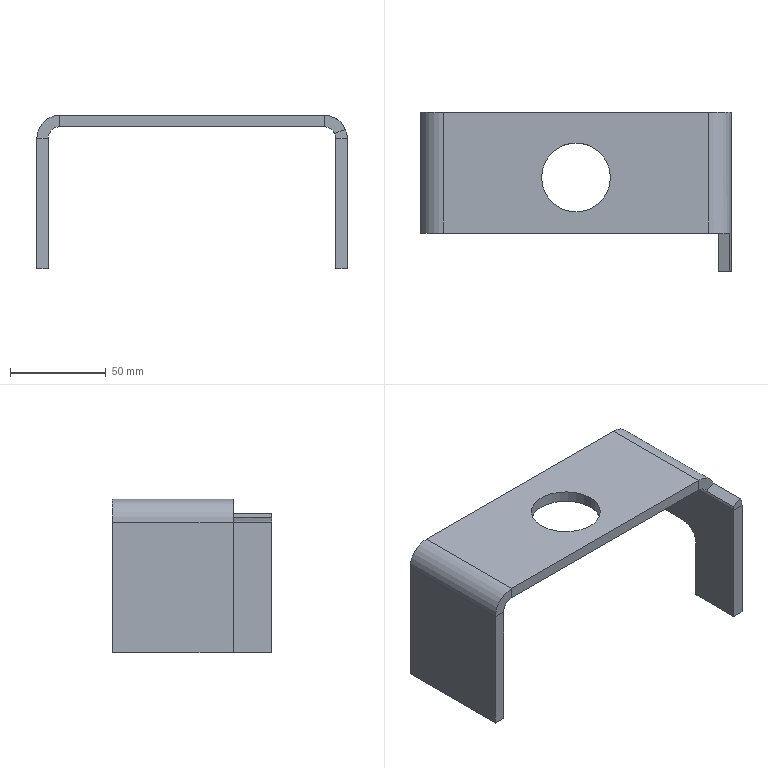Part | SolidWorks | features ICE 3, Fillet 1, FlatPattern 1, SMBaseFlange 1, SheetMetal 1 | 1 solid | 29 faces | box 162 x 83 x 80 mm | volume 102695 mm3 | plane 22 | cylinder 7 | commonest cylinder face diameters 12 x2 24 x2 36 x2 20 x1
STEP:
#1=CARTESIAN_POINT('',(63.,49.,-6.));
#2=VERTEX_POINT('',#1);
#3=CARTESIAN_POINT('',(99.,49.,-6.));
#4=VERTEX_POINT('',#3);
#5=CARTESIAN_POINT('',(81.,49.,-6.));
#6=DIRECTION('',(0.,0.,1.));
#7=DIRECTION('',(1.,0.,0.));
#8=AXIS2_PLACEMENT_3D('',#5,#6,#7);
#9=CIRCLE('',#8,18.);
#10=EDGE_CURVE('',#2,#4,#9,.T.);
#11=ORIENTED_EDGE('',*,*,#10,.F.);
#12=CARTESIAN_POINT('',(63.,49.,0.));
#13=VERTEX_POINT('',#12);
#14=CARTESIAN_POINT('',(63.,49.,-6.));
#15=DIRECTION('',(0.,0.,1.));
#16=VECTOR('',#15,1000.);
#17=LINE('',#14,#16);
#18=EDGE_CURVE('',#2,#13,#17,.T.);
#19=ORIENTED_EDGE('',*,*,#18,.T.);
#20=CARTESIAN_POINT('',(99.,49.,0.));
#21=VERTEX_POINT('',#20);
#22=CARTESIAN_POINT('',(81.,49.,0.));
#23=DIRECTION('',(0.,0.,1.));
#24=DIRECTION('',(1.,0.,0.));
#25=AXIS2_PLACEMENT_3D('',#22,#23,#24);
#26=CIRCLE('',#25,18.);
#27=EDGE_CURVE('',#13,#21,#26,.T.);
#28=ORIENTED_EDGE('',*,*,#27,.T.);
#29=CARTESIAN_POINT('',(99.,49.,-6.));
#30=DIRECTION('',(0.,0.,1.));
#31=VECTOR('',#30,1000.);
#32=LINE('',#29,#31);
#33=EDGE_CURVE('',#4,#21,#32,.T.);
#34=ORIENTED_EDGE('',*,*,#33,.F.);
#35=EDGE_LOOP('',(#11,#19,#28,#34));
#36=FACE_OUTER_BOUND('',#35,.T.);
#37=CARTESIAN_POINT('',(81.,49.,-6.));
#38=DIRECTION('',(0.,0.,1.));
#39=DIRECTION('',(1.,0.,0.));
#40=AXIS2_PLACEMENT_3D('',#37,#38,#39);
#41=CYLINDRICAL_SURFACE('',#40,18.);
#42=ADVANCED_FACE('',(#36),#41,.F.);
#43=CARTESIAN_POINT('',(161.,0.,-7.204));
#44=VERTEX_POINT('',#43);
#45=CARTESIAN_POINT('',(162.,0.,-12.));
#46=VERTEX_POINT('',#45);
#47=CARTESIAN_POINT('',(150.,0.,-12.));
#48=DIRECTION('',(0.,1.,0.));
#49=DIRECTION('',(0.,0.,-1.));
#50=AXIS2_PLACEMENT_3D('',#47,#48,#49);
#51=CIRCLE('',#50,12.);
#52=EDGE_CURVE('',#44,#46,#51,.T.);
#53=ORIENTED_EDGE('',*,*,#52,.F.);
#54=CARTESIAN_POINT('',(155.5,0.,-9.602));
#55=VERTEX_POINT('',#54);
#56=CARTESIAN_POINT('',(155.5,0.,-9.602));
#57=DIRECTION('',(0.9167,0.,0.3997));
#58=VECTOR('',#57,1000.);
#59=LINE('',#56,#58);
#60=EDGE_CURVE('',#55,#44,#59,.T.);
#61=ORIENTED_EDGE('',*,*,#60,.F.);
#62=CARTESIAN_POINT('',(156.,0.,-12.));
#63=VERTEX_POINT('',#62);
#64=CARTESIAN_POINT('',(150.,0.,-12.));
#65=DIRECTION('',(0.,1.,0.));
#66=DIRECTION('',(1.,0.,0.));
#67=AXIS2_PLACEMENT_3D('',#64,#65,#66);
#68=CIRCLE('',#67,6.);
#69=EDGE_CURVE('',#55,#63,#68,.T.);
#70=ORIENTED_EDGE('',*,*,#69,.T.);
#71=CARTESIAN_POINT('',(162.,0.,-12.));
#72=DIRECTION('',(-1.,0.,0.));
#73=VECTOR('',#72,1000.);
#74=LINE('',#71,#73);
#75=EDGE_CURVE('',#46,#63,#74,.T.);
#76=ORIENTED_EDGE('',*,*,#75,.F.);
#77=EDGE_LOOP('',(#53,#61,#70,#76));
#78=FACE_OUTER_BOUND('',#77,.T.);
#79=CARTESIAN_POINT('',(162.,0.,-12.));
#80=DIRECTION('',(0.,-1.,0.));
#81=DIRECTION('',(0.,0.,-1.));
#82=AXIS2_PLACEMENT_3D('',#79,#80,#81);
#83=PLANE('',#82);
#84=ADVANCED_FACE('',(#78),#83,.T.);
#85=CARTESIAN_POINT('',(155.5,20.,-9.602));
#86=VERTEX_POINT('',#85);
#87=CARTESIAN_POINT('',(155.5,83.,-9.602));
#88=DIRECTION('',(0.,-1.,0.));
#89=VECTOR('',#88,1000.);
#90=LINE('',#87,#89);
#91=EDGE_CURVE('',#86,#55,#90,.T.);
#92=ORIENTED_EDGE('',*,*,#91,.F.);
#93=CARTESIAN_POINT('',(150.,20.,-6.));
#94=VERTEX_POINT('',#93);
#95=CARTESIAN_POINT('',(150.,20.,-12.));
#96=DIRECTION('',(0.,-1.,0.));
#97=DIRECTION('',(0.,0.,-1.));
#98=AXIS2_PLACEMENT_3D('',#95,#96,#97);
#99=CIRCLE('',#98,6.);
#100=EDGE_CURVE('',#86,#94,#99,.T.);
#101=ORIENTED_EDGE('',*,*,#100,.T.);
#102=CARTESIAN_POINT('',(150.,83.,-6.));
#103=VERTEX_POINT('',#102);
#104=CARTESIAN_POINT('',(150.,83.,-6.));
#105=DIRECTION('',(0.,-1.,0.));
#106=VECTOR('',#105,1000.);
#107=LINE('',#104,#106);
#108=EDGE_CURVE('',#103,#94,#107,.T.);
#109=ORIENTED_EDGE('',*,*,#108,.F.);
#110=CARTESIAN_POINT('',(156.,83.,-12.));
#111=VERTEX_POINT('',#110);
#112=CARTESIAN_POINT('',(150.,83.,-12.));
#113=DIRECTION('',(0.,1.,0.));
#114=DIRECTION('',(1.,0.,0.));
#115=AXIS2_PLACEMENT_3D('',#112,#113,#114);
#116=CIRCLE('',#115,6.);
#117=EDGE_CURVE('',#103,#111,#116,.T.);
#118=ORIENTED_EDGE('',*,*,#117,.T.);
#119=CARTESIAN_POINT('',(156.,83.,-12.));
#120=DIRECTION('',(0.,-1.,0.));
#121=VECTOR('',#120,1000.);
#122=LINE('',#119,#121);
#123=EDGE_CURVE('',#111,#63,#122,.T.);
#124=ORIENTED_EDGE('',*,*,#123,.T.);
#125=ORIENTED_EDGE('',*,*,#69,.F.);
#126=EDGE_LOOP('',(#92,#101,#109,#118,#124,#125));
#127=FACE_OUTER_BOUND('',#126,.T.);
#128=CARTESIAN_POINT('',(150.,83.,-12.));
#129=DIRECTION('',(0.,-1.,0.));
#130=DIRECTION('',(0.,0.,-1.));
#131=AXIS2_PLACEMENT_3D('',#128,#129,#130);
#132=CYLINDRICAL_SURFACE('',#131,6.);
#133=ADVANCED_FACE('',(#127),#132,.F.);
#134=CARTESIAN_POINT('',(81.,49.,-6.));
#135=DIRECTION('',(0.,0.,1.));
#136=DIRECTION('',(1.,0.,0.));
#137=AXIS2_PLACEMENT_3D('',#134,#135,#136);
#138=CIRCLE('',#137,18.);
#139=EDGE_CURVE('',#4,#2,#138,.T.);
#140=ORIENTED_EDGE('',*,*,#139,.T.);
#141=ORIENTED_EDGE('',*,*,#10,.T.);
#142=EDGE_LOOP('',(#140,#141));
#143=FACE_BOUND('',#142,.T.);
#144=ORIENTED_EDGE('',*,*,#108,.T.);
#145=CARTESIAN_POINT('',(12.,20.,-6.));
#146=VERTEX_POINT('',#145);
#147=CARTESIAN_POINT('',(0.,20.,-6.));
#148=DIRECTION('',(-1.,0.,0.));
#149=VECTOR('',#148,1000.);
#150=LINE('',#147,#149);
#151=EDGE_CURVE('',#94,#146,#150,.T.);
#152=ORIENTED_EDGE('',*,*,#151,.T.);
#153=CARTESIAN_POINT('',(12.,83.,-6.));
#154=VERTEX_POINT('',#153);
#155=CARTESIAN_POINT('',(12.,83.,-6.));
#156=DIRECTION('',(0.,-1.,0.));
#157=VECTOR('',#156,1000.);
#158=LINE('',#155,#157);
#159=EDGE_CURVE('',#154,#146,#158,.T.);
#160=ORIENTED_EDGE('',*,*,#159,.F.);
#161=CARTESIAN_POINT('',(0.,83.,-6.));
#162=DIRECTION('',(1.,0.,0.));
#163=VECTOR('',#162,1000.);
#164=LINE('',#161,#163);
#165=EDGE_CURVE('',#154,#103,#164,.T.);
#166=ORIENTED_EDGE('',*,*,#165,.T.);
#167=EDGE_LOOP('',(#144,#152,#160,#166));
#168=FACE_OUTER_BOUND('',#167,.T.);
#169=CARTESIAN_POINT('',(0.,83.,-6.));
#170=DIRECTION('',(0.,0.,-1.));
#171=DIRECTION('',(-1.,0.,0.));
#172=AXIS2_PLACEMENT_3D('',#169,#170,#171);
#173=PLANE('',#172);
#174=ADVANCED_FACE('',(#143,#168),#173,.T.);
#175=ORIENTED_EDGE('',*,*,#159,.T.);
#176=CARTESIAN_POINT('',(6.,20.,-12.));
#177=VERTEX_POINT('',#176);
#178=CARTESIAN_POINT('',(12.,20.,-12.));
#179=DIRECTION('',(0.,-1.,0.));
#180=DIRECTION('',(0.,0.,-1.));
#181=AXIS2_PLACEMENT_3D('',#178,#179,#180);
#182=CIRCLE('',#181,6.);
#183=EDGE_CURVE('',#146,#177,#182,.T.);
#184=ORIENTED_EDGE('',*,*,#183,.T.);
#185=CARTESIAN_POINT('',(6.,83.,-12.));
#186=VERTEX_POINT('',#185);
#187=CARTESIAN_POINT('',(6.,83.,-12.));
#188=DIRECTION('',(0.,-1.,0.));
#189=VECTOR('',#188,1000.);
#190=LINE('',#187,#189);
#191=EDGE_CURVE('',#186,#177,#190,.T.);
#192=ORIENTED_EDGE('',*,*,#191,.F.);
#193=CARTESIAN_POINT('',(12.,83.,-12.));
#194=DIRECTION('',(0.,1.,0.));
#195=DIRECTION('',(1.,0.,0.));
#196=AXIS2_PLACEMENT_3D('',#193,#194,#195);
#197=CIRCLE('',#196,6.);
#198=EDGE_CURVE('',#186,#154,#197,.T.);
#199=ORIENTED_EDGE('',*,*,#198,.T.);
#200=EDGE_LOOP('',(#175,#184,#192,#199));
#201=FACE_OUTER_BOUND('',#200,.T.);
#202=CARTESIAN_POINT('',(12.,83.,-12.));
#203=DIRECTION('',(0.,-1.,0.));
#204=DIRECTION('',(0.,0.,-1.));
#205=AXIS2_PLACEMENT_3D('',#202,#203,#204);
#206=CYLINDRICAL_SURFACE('',#205,6.);
#207=ADVANCED_FACE('',(#201),#206,.F.);
#208=ORIENTED_EDGE('',*,*,#191,.T.);
#209=CARTESIAN_POINT('',(6.,20.,-80.));
#210=VERTEX_POINT('',#209);
#211=CARTESIAN_POINT('',(6.,20.,-80.));
#212=DIRECTION('',(0.,0.,-1.));
#213=VECTOR('',#212,1000.);
#214=LINE('',#211,#213);
#215=EDGE_CURVE('',#177,#210,#214,.T.);
#216=ORIENTED_EDGE('',*,*,#215,.T.);
#217=CARTESIAN_POINT('',(6.,83.,-80.));
#218=VERTEX_POINT('',#217);
#219=CARTESIAN_POINT('',(6.,83.,-80.));
#220=DIRECTION('',(0.,-1.,0.));
#221=VECTOR('',#220,1000.);
#222=LINE('',#219,#221);
#223=EDGE_CURVE('',#218,#210,#222,.T.);
#224=ORIENTED_EDGE('',*,*,#223,.F.);
#225=CARTESIAN_POINT('',(6.,83.,-80.));
#226=DIRECTION('',(0.,0.,1.));
#227=VECTOR('',#226,1000.);
#228=LINE('',#225,#227);
#229=EDGE_CURVE('',#218,#186,#228,.T.);
#230=ORIENTED_EDGE('',*,*,#229,.T.);
#231=EDGE_LOOP('',(#208,#216,#224,#230));
#232=FACE_OUTER_BOUND('',#231,.T.);
#233=CARTESIAN_POINT('',(6.,83.,-80.));
#234=DIRECTION('',(1.,0.,0.));
#235=DIRECTION('',(0.,0.,-1.));
#236=AXIS2_PLACEMENT_3D('',#233,#234,#235);
#237=PLANE('',#236);
#238=ADVANCED_FACE('',(#232),#237,.T.);
#239=ORIENTED_EDGE('',*,*,#223,.T.);
#240=CARTESIAN_POINT('',(0.,20.,-80.));
#241=VERTEX_POINT('',#240);
#242=CARTESIAN_POINT('',(6.,20.,-80.));
#243=DIRECTION('',(-1.,0.,0.));
#244=VECTOR('',#243,1000.);
#245=LINE('',#242,#244);
#246=EDGE_CURVE('',#210,#241,#245,.T.);
#247=ORIENTED_EDGE('',*,*,#246,.T.);
#248=CARTESIAN_POINT('',(0.,83.,-80.));
#249=VERTEX_POINT('',#248);
#250=CARTESIAN_POINT('',(0.,83.,-80.));
#251=DIRECTION('',(0.,-1.,0.));
#252=VECTOR('',#251,1000.);
#253=LINE('',#250,#252);
#254=EDGE_CURVE('',#249,#241,#253,.T.);
#255=ORIENTED_EDGE('',*,*,#254,.F.);
#256=CARTESIAN_POINT('',(0.,83.,-80.));
#257=DIRECTION('',(1.,0.,0.));
#258=VECTOR('',#257,1000.);
#259=LINE('',#256,#258);
#260=EDGE_CURVE('',#249,#218,#259,.T.);
#261=ORIENTED_EDGE('',*,*,#260,.T.);
#262=EDGE_LOOP('',(#239,#247,#255,#261));
#263=FACE_OUTER_BOUND('',#262,.T.);
#264=CARTESIAN_POINT('',(0.,83.,-80.));
#265=DIRECTION('',(0.,0.,-1.));
#266=DIRECTION('',(-1.,0.,0.));
#267=AXIS2_PLACEMENT_3D('',#264,#265,#266);
#268=PLANE('',#267);
#269=ADVANCED_FACE('',(#263),#268,.T.);
#270=CARTESIAN_POINT('',(0.,20.,-12.));
#271=VERTEX_POINT('',#270);
#272=CARTESIAN_POINT('',(0.,20.,-80.));
#273=DIRECTION('',(0.,0.,-1.));
#274=VECTOR('',#273,1000.);
#275=LINE('',#272,#274);
#276=EDGE_CURVE('',#271,#241,#275,.T.);
#277=ORIENTED_EDGE('',*,*,#276,.F.);
#278=CARTESIAN_POINT('',(0.,83.,-12.));
#279=VERTEX_POINT('',#278);
#280=CARTESIAN_POINT('',(0.,83.,-12.));
#281=DIRECTION('',(0.,-1.,0.));
#282=VECTOR('',#281,1000.);
#283=LINE('',#280,#282);
#284=EDGE_CURVE('',#279,#271,#283,.T.);
#285=ORIENTED_EDGE('',*,*,#284,.F.);
#286=CARTESIAN_POINT('',(0.,83.,-80.));
#287=DIRECTION('',(0.,0.,1.));
#288=VECTOR('',#287,1000.);
#289=LINE('',#286,#288);
#290=EDGE_CURVE('',#249,#279,#289,.T.);
#291=ORIENTED_EDGE('',*,*,#290,.F.);
#292=ORIENTED_EDGE('',*,*,#254,.T.);
#293=EDGE_LOOP('',(#277,#285,#291,#292));
#294=FACE_OUTER_BOUND('',#293,.T.);
#295=CARTESIAN_POINT('',(0.,83.,-80.));
#296=DIRECTION('',(1.,0.,0.));
#297=DIRECTION('',(0.,0.,-1.));
#298=AXIS2_PLACEMENT_3D('',#295,#296,#297);
#299=PLANE('',#298);
#300=ADVANCED_FACE('',(#294),#299,.F.);
#301=CARTESIAN_POINT('',(12.,20.,0.));
#302=VERTEX_POINT('',#301);
#303=CARTESIAN_POINT('',(12.,20.,-12.));
#304=DIRECTION('',(0.,-1.,0.));
#305=DIRECTION('',(0.,0.,-1.));
#306=AXIS2_PLACEMENT_3D('',#303,#304,#305);
#307=CIRCLE('',#306,12.);
#308=EDGE_CURVE('',#302,#271,#307,.T.);
#309=ORIENTED_EDGE('',*,*,#308,.F.);
#310=CARTESIAN_POINT('',(12.,83.,0.));
#311=VERTEX_POINT('',#310);
#312=CARTESIAN_POINT('',(12.,83.,0.));
#313=DIRECTION('',(0.,-1.,0.));
#314=VECTOR('',#313,1000.);
#315=LINE('',#312,#314);
#316=EDGE_CURVE('',#311,#302,#315,.T.);
#317=ORIENTED_EDGE('',*,*,#316,.F.);
#318=CARTESIAN_POINT('',(12.,83.,-12.));
#319=DIRECTION('',(0.,1.,0.));
#320=DIRECTION('',(0.,0.,-1.));
#321=AXIS2_PLACEMENT_3D('',#318,#319,#320);
#322=CIRCLE('',#321,12.);
#323=EDGE_CURVE('',#279,#311,#322,.T.);
#324=ORIENTED_EDGE('',*,*,#323,.F.);
#325=ORIENTED_EDGE('',*,*,#284,.T.);
#326=EDGE_LOOP('',(#309,#317,#324,#325));
#327=FACE_OUTER_BOUND('',#326,.T.);
#328=CARTESIAN_POINT('',(12.,83.,-12.));
#329=DIRECTION('',(0.,-1.,0.));
#330=DIRECTION('',(0.,0.,-1.));
#331=AXIS2_PLACEMENT_3D('',#328,#329,#330);
#332=CYLINDRICAL_SURFACE('',#331,12.);
#333=ADVANCED_FACE('',(#327),#332,.T.);
#334=CARTESIAN_POINT('',(81.,49.,0.));
#335=DIRECTION('',(0.,0.,1.));
#336=DIRECTION('',(1.,0.,0.));
#337=AXIS2_PLACEMENT_3D('',#334,#335,#336);
#338=CIRCLE('',#337,18.);
#339=EDGE_CURVE('',#21,#13,#338,.T.);
#340=ORIENTED_EDGE('',*,*,#339,.F.);
#341=ORIENTED_EDGE('',*,*,#27,.F.);
#342=EDGE_LOOP('',(#340,#341));
#343=FACE_BOUND('',#342,.T.);
#344=CARTESIAN_POINT('',(150.,20.,0.));
#345=VERTEX_POINT('',#344);
#346=CARTESIAN_POINT('',(0.,20.,0.));
#347=DIRECTION('',(-1.,0.,0.));
#348=VECTOR('',#347,1000.);
#349=LINE('',#346,#348);
#350=EDGE_CURVE('',#345,#302,#349,.T.);
#351=ORIENTED_EDGE('',*,*,#350,.F.);
#352=CARTESIAN_POINT('',(150.,83.,0.));
#353=VERTEX_POINT('',#352);
#354=CARTESIAN_POINT('',(150.,83.,0.));
#355=DIRECTION('',(0.,-1.,0.));
#356=VECTOR('',#355,1000.);
#357=LINE('',#354,#356);
#358=EDGE_CURVE('',#353,#345,#357,.T.);
#359=ORIENTED_EDGE('',*,*,#358,.F.);
#360=CARTESIAN_POINT('',(0.,83.,0.));
#361=DIRECTION('',(1.,0.,0.));
#362=VECTOR('',#361,1000.);
#363=LINE('',#360,#362);
#364=EDGE_CURVE('',#311,#353,#363,.T.);
#365=ORIENTED_EDGE('',*,*,#364,.F.);
#366=ORIENTED_EDGE('',*,*,#316,.T.);
#367=EDGE_LOOP('',(#351,#359,#365,#366));
#368=FACE_OUTER_BOUND('',#367,.T.);
#369=CARTESIAN_POINT('',(0.,83.,0.));
#370=DIRECTION('',(0.,0.,-1.));
#371=DIRECTION('',(-1.,0.,0.));
#372=AXIS2_PLACEMENT_3D('',#369,#370,#371);
#373=PLANE('',#372);
#374=ADVANCED_FACE('',(#343,#368),#373,.F.);
#375=CARTESIAN_POINT('',(161.,20.,-7.204));
#376=VERTEX_POINT('',#375);
#377=CARTESIAN_POINT('',(150.,20.,-12.));
#378=DIRECTION('',(0.,-1.,0.));
#379=DIRECTION('',(0.,0.,-1.));
#380=AXIS2_PLACEMENT_3D('',#377,#378,#379);
#381=CIRCLE('',#380,12.);
#382=EDGE_CURVE('',#376,#345,#381,.T.);
#383=ORIENTED_EDGE('',*,*,#382,.F.);
#384=CARTESIAN_POINT('',(161.,83.,-7.204));
#385=DIRECTION('',(0.,-1.,0.));
#386=VECTOR('',#385,1000.);
#387=LINE('',#384,#386);
#388=EDGE_CURVE('',#376,#44,#387,.T.);
#389=ORIENTED_EDGE('',*,*,#388,.T.);
#390=ORIENTED_EDGE('',*,*,#52,.T.);
#391=CARTESIAN_POINT('',(162.,83.,-12.));
#392=VERTEX_POINT('',#391);
#393=CARTESIAN_POINT('',(162.,83.,-12.));
#394=DIRECTION('',(0.,-1.,0.));
#395=VECTOR('',#394,1000.);
#396=LINE('',#393,#395);
#397=EDGE_CURVE('',#392,#46,#396,.T.);
#398=ORIENTED_EDGE('',*,*,#397,.F.);
#399=CARTESIAN_POINT('',(150.,83.,-12.));
#400=DIRECTION('',(0.,1.,0.));
#401=DIRECTION('',(0.,0.,-1.));
#402=AXIS2_PLACEMENT_3D('',#399,#400,#401);
#403=CIRCLE('',#402,12.);
#404=EDGE_CURVE('',#353,#392,#403,.T.);
#405=ORIENTED_EDGE('',*,*,#404,.F.);
#406=ORIENTED_EDGE('',*,*,#358,.T.);
#407=EDGE_LOOP('',(#383,#389,#390,#398,#405,#406));
#408=FACE_OUTER_BOUND('',#407,.T.);
#409=CARTESIAN_POINT('',(150.,83.,-12.));
#410=DIRECTION('',(0.,-1.,0.));
#411=DIRECTION('',(0.,0.,-1.));
#412=AXIS2_PLACEMENT_3D('',#409,#410,#411);
#413=CYLINDRICAL_SURFACE('',#412,12.);
#414=ADVANCED_FACE('',(#408),#413,.T.);
#415=CARTESIAN_POINT('',(0.,83.,-12.));
#416=DIRECTION('',(1.,0.,0.));
#417=VECTOR('',#416,1000.);
#418=LINE('',#415,#417);
#419=EDGE_CURVE('',#279,#186,#418,.T.);
#420=ORIENTED_EDGE('',*,*,#419,.F.);
#421=ORIENTED_EDGE('',*,*,#323,.T.);
#422=CARTESIAN_POINT('',(12.,83.,-6.));
#423=DIRECTION('',(0.,0.,1.));
#424=VECTOR('',#423,1000.);
#425=LINE('',#422,#424);
#426=EDGE_CURVE('',#154,#311,#425,.T.);
#427=ORIENTED_EDGE('',*,*,#426,.F.);
#428=ORIENTED_EDGE('',*,*,#198,.F.);
#429=EDGE_LOOP('',(#420,#421,#427,#428));
#430=FACE_OUTER_BOUND('',#429,.T.);
#431=CARTESIAN_POINT('',(0.,83.,-12.));
#432=DIRECTION('',(0.,1.,0.));
#433=DIRECTION('',(0.,0.,1.));
#434=AXIS2_PLACEMENT_3D('',#431,#432,#433);
#435=PLANE('',#434);
#436=ADVANCED_FACE('',(#430),#435,.T.);
#437=ORIENTED_EDGE('',*,*,#290,.T.);
#438=ORIENTED_EDGE('',*,*,#419,.T.);
#439=ORIENTED_EDGE('',*,*,#229,.F.);
#440=ORIENTED_EDGE('',*,*,#260,.F.);
#441=EDGE_LOOP('',(#437,#438,#439,#440));
#442=FACE_OUTER_BOUND('',#441,.T.);
#443=CARTESIAN_POINT('',(12.,83.,-6.));
#444=DIRECTION('',(0.,1.,0.));
#445=DIRECTION('',(0.,0.,1.));
#446=AXIS2_PLACEMENT_3D('',#443,#444,#445);
#447=PLANE('',#446);
#448=ADVANCED_FACE('',(#442),#447,.T.);
#449=CARTESIAN_POINT('',(150.,83.,0.));
#450=DIRECTION('',(0.,0.,-1.));
#451=VECTOR('',#450,1000.);
#452=LINE('',#449,#451);
#453=EDGE_CURVE('',#353,#103,#452,.T.);
#454=ORIENTED_EDGE('',*,*,#453,.F.);
#455=ORIENTED_EDGE('',*,*,#404,.T.);
#456=CARTESIAN_POINT('',(156.,83.,-12.));
#457=DIRECTION('',(1.,0.,0.));
#458=VECTOR('',#457,1000.);
#459=LINE('',#456,#458);
#460=EDGE_CURVE('',#111,#392,#459,.T.);
#461=ORIENTED_EDGE('',*,*,#460,.F.);
#462=ORIENTED_EDGE('',*,*,#117,.F.);
#463=EDGE_LOOP('',(#454,#455,#461,#462));
#464=FACE_OUTER_BOUND('',#463,.T.);
#465=CARTESIAN_POINT('',(150.,83.,0.));
#466=DIRECTION('',(0.,1.,0.));
#467=DIRECTION('',(0.,0.,1.));
#468=AXIS2_PLACEMENT_3D('',#465,#466,#467);
#469=PLANE('',#468);
#470=ADVANCED_FACE('',(#464),#469,.T.);
#471=ORIENTED_EDGE('',*,*,#364,.T.);
#472=ORIENTED_EDGE('',*,*,#453,.T.);
#473=ORIENTED_EDGE('',*,*,#165,.F.);
#474=ORIENTED_EDGE('',*,*,#426,.T.);
#475=EDGE_LOOP('',(#471,#472,#473,#474));
#476=FACE_OUTER_BOUND('',#475,.T.);
#477=CARTESIAN_POINT('',(156.,83.,-12.));
#478=DIRECTION('',(0.,1.,0.));
#479=DIRECTION('',(0.,0.,1.));
#480=AXIS2_PLACEMENT_3D('',#477,#478,#479);
#481=PLANE('',#480);
#482=ADVANCED_FACE('',(#476),#481,.T.);
#483=CARTESIAN_POINT('',(162.,0.,-80.));
#484=VERTEX_POINT('',#483);
#485=CARTESIAN_POINT('',(162.,0.,0.));
#486=DIRECTION('',(0.,0.,-1.));
#487=VECTOR('',#486,1000.);
#488=LINE('',#485,#487);
#489=EDGE_CURVE('',#46,#484,#488,.T.);
#490=ORIENTED_EDGE('',*,*,#489,.F.);
#491=ORIENTED_EDGE('',*,*,#75,.T.);
#492=CARTESIAN_POINT('',(156.,0.,-80.));
#493=VERTEX_POINT('',#492);
#494=CARTESIAN_POINT('',(156.,0.,0.));
#495=DIRECTION('',(0.,0.,-1.));
#496=VECTOR('',#495,1000.);
#497=LINE('',#494,#496);
#498=EDGE_CURVE('',#63,#493,#497,.T.);
#499=ORIENTED_EDGE('',*,*,#498,.T.);
#500=CARTESIAN_POINT('',(156.,0.,-80.));
#501=DIRECTION('',(1.,0.,0.));
#502=VECTOR('',#501,1000.);
#503=LINE('',#500,#502);
#504=EDGE_CURVE('',#493,#484,#503,.T.);
#505=ORIENTED_EDGE('',*,*,#504,.T.);
#506=EDGE_LOOP('',(#490,#491,#499,#505));
#507=FACE_OUTER_BOUND('',#506,.T.);
#508=CARTESIAN_POINT('',(150.,0.,-6.));
#509=DIRECTION('',(0.,-1.,0.));
#510=DIRECTION('',(0.,0.,-1.));
#511=AXIS2_PLACEMENT_3D('',#508,#509,#510);
#512=PLANE('',#511);
#513=ADVANCED_FACE('',(#507),#512,.T.);
#514=CARTESIAN_POINT('',(162.,28.,-80.));
#515=VERTEX_POINT('',#514);
#516=CARTESIAN_POINT('',(162.,28.,-47.));
#517=VERTEX_POINT('',#516);
#518=CARTESIAN_POINT('',(162.,28.,-80.));
#519=DIRECTION('',(0.,0.,1.));
#520=VECTOR('',#519,1000.);
#521=LINE('',#518,#520);
#522=EDGE_CURVE('',#515,#517,#521,.T.);
#523=ORIENTED_EDGE('',*,*,#522,.T.);
#524=CARTESIAN_POINT('',(162.,38.,-37.));
#525=VERTEX_POINT('',#524);
#526=CARTESIAN_POINT('',(162.,38.,-47.));
#527=DIRECTION('',(-1.,0.,0.));
#528=DIRECTION('',(0.,0.,1.));
#529=AXIS2_PLACEMENT_3D('',#526,#527,#528);
#530=CIRCLE('',#529,10.);
#531=EDGE_CURVE('',#517,#525,#530,.T.);
#532=ORIENTED_EDGE('',*,*,#531,.T.);
#533=CARTESIAN_POINT('',(162.,83.,-37.));
#534=VERTEX_POINT('',#533);
#535=CARTESIAN_POINT('',(162.,28.,-37.));
#536=DIRECTION('',(0.,1.,0.));
#537=VECTOR('',#536,1000.);
#538=LINE('',#535,#537);
#539=EDGE_CURVE('',#525,#534,#538,.T.);
#540=ORIENTED_EDGE('',*,*,#539,.T.);
#541=CARTESIAN_POINT('',(162.,83.,0.));
#542=DIRECTION('',(0.,0.,-1.));
#543=VECTOR('',#542,1000.);
#544=LINE('',#541,#543);
#545=EDGE_CURVE('',#392,#534,#544,.T.);
#546=ORIENTED_EDGE('',*,*,#545,.F.);
#547=ORIENTED_EDGE('',*,*,#397,.T.);
#548=ORIENTED_EDGE('',*,*,#489,.T.);
#549=CARTESIAN_POINT('',(162.,83.,-80.));
#550=DIRECTION('',(0.,-1.,0.));
#551=VECTOR('',#550,1000.);
#552=LINE('',#549,#551);
#553=EDGE_CURVE('',#515,#484,#552,.T.);
#554=ORIENTED_EDGE('',*,*,#553,.F.);
#555=EDGE_LOOP('',(#523,#532,#540,#546,#547,#548,#554));
#556=FACE_OUTER_BOUND('',#555,.T.);
#557=CARTESIAN_POINT('',(162.,83.,0.));
#558=DIRECTION('',(-1.,0.,0.));
#559=DIRECTION('',(0.,0.,1.));
#560=AXIS2_PLACEMENT_3D('',#557,#558,#559);
#561=PLANE('',#560);
#562=ADVANCED_FACE('',(#556),#561,.F.);
#563=CARTESIAN_POINT('',(156.,28.,-80.));
#564=VERTEX_POINT('',#563);
#565=CARTESIAN_POINT('',(162.,28.,-80.));
#566=DIRECTION('',(-1.,0.,0.));
#567=VECTOR('',#566,1000.);
#568=LINE('',#565,#567);
#569=EDGE_CURVE('',#515,#564,#568,.T.);
#570=ORIENTED_EDGE('',*,*,#569,.F.);
#571=ORIENTED_EDGE('',*,*,#553,.T.);
#572=ORIENTED_EDGE('',*,*,#504,.F.);
#573=CARTESIAN_POINT('',(156.,83.,-80.));
#574=DIRECTION('',(0.,-1.,0.));
#575=VECTOR('',#574,1000.);
#576=LINE('',#573,#575);
#577=EDGE_CURVE('',#564,#493,#576,.T.);
#578=ORIENTED_EDGE('',*,*,#577,.F.);
#579=EDGE_LOOP('',(#570,#571,#572,#578));
#580=FACE_OUTER_BOUND('',#579,.T.);
#581=CARTESIAN_POINT('',(156.,83.,-80.));
#582=DIRECTION('',(0.,0.,-1.));
#583=DIRECTION('',(-1.,0.,0.));
#584=AXIS2_PLACEMENT_3D('',#581,#582,#583);
#585=PLANE('',#584);
#586=ADVANCED_FACE('',(#580),#585,.T.);
#587=CARTESIAN_POINT('',(156.,38.,-37.));
#588=VERTEX_POINT('',#587);
#589=CARTESIAN_POINT('',(156.,83.,-37.));
#590=VERTEX_POINT('',#589);
#591=CARTESIAN_POINT('',(156.,28.,-37.));
#592=DIRECTION('',(0.,1.,0.));
#593=VECTOR('',#592,1000.);
#594=LINE('',#591,#593);
#595=EDGE_CURVE('',#588,#590,#594,.T.);
#596=ORIENTED_EDGE('',*,*,#595,.F.);
#597=CARTESIAN_POINT('',(156.,28.,-47.));
#598=VERTEX_POINT('',#597);
#599=CARTESIAN_POINT('',(156.,38.,-47.));
#600=DIRECTION('',(1.,0.,0.));
#601=DIRECTION('',(0.,0.,1.));
#602=AXIS2_PLACEMENT_3D('',#599,#600,#601);
#603=CIRCLE('',#602,10.);
#604=EDGE_CURVE('',#588,#598,#603,.T.);
#605=ORIENTED_EDGE('',*,*,#604,.T.);
#606=CARTESIAN_POINT('',(156.,28.,-80.));
#607=DIRECTION('',(0.,0.,1.));
#608=VECTOR('',#607,1000.);
#609=LINE('',#606,#608);
#610=EDGE_CURVE('',#564,#598,#609,.T.);
#611=ORIENTED_EDGE('',*,*,#610,.F.);
#612=ORIENTED_EDGE('',*,*,#577,.T.);
#613=ORIENTED_EDGE('',*,*,#498,.F.);
#614=ORIENTED_EDGE('',*,*,#123,.F.);
#615=CARTESIAN_POINT('',(156.,83.,0.));
#616=DIRECTION('',(0.,0.,-1.));
#617=VECTOR('',#616,1000.);
#618=LINE('',#615,#617);
#619=EDGE_CURVE('',#111,#590,#618,.T.);
#620=ORIENTED_EDGE('',*,*,#619,.T.);
#621=EDGE_LOOP('',(#596,#605,#611,#612,#613,#614,#620));
#622=FACE_OUTER_BOUND('',#621,.T.);
#623=CARTESIAN_POINT('',(156.,83.,0.));
#624=DIRECTION('',(-1.,0.,0.));
#625=DIRECTION('',(0.,0.,1.));
#626=AXIS2_PLACEMENT_3D('',#623,#624,#625);
#627=PLANE('',#626);
#628=ADVANCED_FACE('',(#622),#627,.T.);
#629=CARTESIAN_POINT('',(162.,83.,-37.));
#630=DIRECTION('',(-1.,0.,0.));
#631=VECTOR('',#630,1000.);
#632=LINE('',#629,#631);
#633=EDGE_CURVE('',#534,#590,#632,.T.);
#634=ORIENTED_EDGE('',*,*,#633,.T.);
#635=ORIENTED_EDGE('',*,*,#619,.F.);
#636=ORIENTED_EDGE('',*,*,#460,.T.);
#637=ORIENTED_EDGE('',*,*,#545,.T.);
#638=EDGE_LOOP('',(#634,#635,#636,#637));
#639=FACE_OUTER_BOUND('',#638,.T.);
#640=CARTESIAN_POINT('',(150.,83.,-12.));
#641=DIRECTION('',(0.,1.,0.));
#642=DIRECTION('',(1.,0.,0.));
#643=AXIS2_PLACEMENT_3D('',#640,#641,#642);
#644=PLANE('',#643);
#645=ADVANCED_FACE('',(#639),#644,.T.);
#646=ORIENTED_EDGE('',*,*,#246,.F.);
#647=ORIENTED_EDGE('',*,*,#215,.F.);
#648=CARTESIAN_POINT('',(6.,20.,-12.));
#649=DIRECTION('',(-1.,0.,0.));
#650=VECTOR('',#649,1000.);
#651=LINE('',#648,#650);
#652=EDGE_CURVE('',#177,#271,#651,.T.);
#653=ORIENTED_EDGE('',*,*,#652,.T.);
#654=ORIENTED_EDGE('',*,*,#276,.T.);
#655=EDGE_LOOP('',(#646,#647,#653,#654));
#656=FACE_OUTER_BOUND('',#655,.T.);
#657=CARTESIAN_POINT('',(6.,20.,-80.));
#658=DIRECTION('',(0.,-1.,0.));
#659=DIRECTION('',(0.,0.,-1.));
#660=AXIS2_PLACEMENT_3D('',#657,#658,#659);
#661=PLANE('',#660);
#662=ADVANCED_FACE('',(#656),#661,.T.);
#663=ORIENTED_EDGE('',*,*,#652,.F.);
#664=ORIENTED_EDGE('',*,*,#183,.F.);
#665=CARTESIAN_POINT('',(12.,20.,-6.));
#666=DIRECTION('',(0.,0.,1.));
#667=VECTOR('',#666,1000.);
#668=LINE('',#665,#667);
#669=EDGE_CURVE('',#146,#302,#668,.T.);
#670=ORIENTED_EDGE('',*,*,#669,.T.);
#671=ORIENTED_EDGE('',*,*,#308,.T.);
#672=EDGE_LOOP('',(#663,#664,#670,#671));
#673=FACE_OUTER_BOUND('',#672,.T.);
#674=CARTESIAN_POINT('',(12.,20.,-12.));
#675=DIRECTION('',(0.,1.,0.));
#676=DIRECTION('',(0.,0.,1.));
#677=AXIS2_PLACEMENT_3D('',#674,#675,#676);
#678=PLANE('',#677);
#679=ADVANCED_FACE('',(#673),#678,.F.);
#680=ORIENTED_EDGE('',*,*,#669,.F.);
#681=ORIENTED_EDGE('',*,*,#151,.F.);
#682=CARTESIAN_POINT('',(150.,20.,-6.));
#683=DIRECTION('',(0.,0.,1.));
#684=VECTOR('',#683,1000.);
#685=LINE('',#682,#684);
#686=EDGE_CURVE('',#94,#345,#685,.T.);
#687=ORIENTED_EDGE('',*,*,#686,.T.);
#688=ORIENTED_EDGE('',*,*,#350,.T.);
#689=EDGE_LOOP('',(#680,#681,#687,#688));
#690=FACE_OUTER_BOUND('',#689,.T.);
#691=CARTESIAN_POINT('',(0.,20.,-6.));
#692=DIRECTION('',(0.,-1.,0.));
#693=DIRECTION('',(-1.,0.,0.));
#694=AXIS2_PLACEMENT_3D('',#691,#692,#693);
#695=PLANE('',#694);
#696=ADVANCED_FACE('',(#690),#695,.T.);
#697=ORIENTED_EDGE('',*,*,#686,.F.);
#698=ORIENTED_EDGE('',*,*,#100,.F.);
#699=CARTESIAN_POINT('',(155.5,20.,-9.602));
#700=DIRECTION('',(0.9167,0.,0.3997));
#701=VECTOR('',#700,1000.);
#702=LINE('',#699,#701);
#703=EDGE_CURVE('',#86,#376,#702,.T.);
#704=ORIENTED_EDGE('',*,*,#703,.T.);
#705=ORIENTED_EDGE('',*,*,#382,.T.);
#706=EDGE_LOOP('',(#697,#698,#704,#705));
#707=FACE_OUTER_BOUND('',#706,.T.);
#708=CARTESIAN_POINT('',(150.,20.,-12.));
#709=DIRECTION('',(0.,1.,0.));
#710=DIRECTION('',(0.,0.,1.));
#711=AXIS2_PLACEMENT_3D('',#708,#709,#710);
#712=PLANE('',#711);
#713=ADVANCED_FACE('',(#707),#712,.F.);
#714=ORIENTED_EDGE('',*,*,#91,.T.);
#715=ORIENTED_EDGE('',*,*,#60,.T.);
#716=ORIENTED_EDGE('',*,*,#388,.F.);
#717=ORIENTED_EDGE('',*,*,#703,.F.);
#718=EDGE_LOOP('',(#714,#715,#716,#717));
#719=FACE_OUTER_BOUND('',#718,.T.);
#720=CARTESIAN_POINT('',(155.5,10.,-9.602));
#721=DIRECTION('',(-0.3997,0.,0.9167));
#722=DIRECTION('',(0.,-1.,0.));
#723=AXIS2_PLACEMENT_3D('',#720,#721,#722);
#724=PLANE('',#723);
#725=ADVANCED_FACE('',(#719),#724,.T.);
#726=ORIENTED_EDGE('',*,*,#539,.F.);
#727=CARTESIAN_POINT('',(156.,38.,-37.));
#728=DIRECTION('',(-1.,0.,0.));
#729=VECTOR('',#728,1000.);
#730=LINE('',#727,#729);
#731=EDGE_CURVE('',#525,#588,#730,.T.);
#732=ORIENTED_EDGE('',*,*,#731,.T.);
#733=ORIENTED_EDGE('',*,*,#595,.T.);
#734=ORIENTED_EDGE('',*,*,#633,.F.);
#735=EDGE_LOOP('',(#726,#732,#733,#734));
#736=FACE_OUTER_BOUND('',#735,.T.);
#737=CARTESIAN_POINT('',(162.,28.,-37.));
#738=DIRECTION('',(0.,0.,1.));
#739=DIRECTION('',(1.,0.,0.));
#740=AXIS2_PLACEMENT_3D('',#737,#738,#739);
#741=PLANE('',#740);
#742=ADVANCED_FACE('',(#736),#741,.F.);
#743=ORIENTED_EDGE('',*,*,#610,.T.);
#744=CARTESIAN_POINT('',(162.,28.,-47.));
#745=DIRECTION('',(1.,0.,0.));
#746=VECTOR('',#745,1000.);
#747=LINE('',#744,#746);
#748=EDGE_CURVE('',#598,#517,#747,.T.);
#749=ORIENTED_EDGE('',*,*,#748,.T.);
#750=ORIENTED_EDGE('',*,*,#522,.F.);
#751=ORIENTED_EDGE('',*,*,#569,.T.);
#752=EDGE_LOOP('',(#743,#749,#750,#751));
#753=FACE_OUTER_BOUND('',#752,.T.);
#754=CARTESIAN_POINT('',(162.,28.,-80.));
#755=DIRECTION('',(0.,-1.,0.));
#756=DIRECTION('',(0.,0.,-1.));
#757=AXIS2_PLACEMENT_3D('',#754,#755,#756);
#758=PLANE('',#757);
#759=ADVANCED_FACE('',(#753),#758,.F.);
#760=ORIENTED_EDGE('',*,*,#531,.F.);
#761=ORIENTED_EDGE('',*,*,#748,.F.);
#762=ORIENTED_EDGE('',*,*,#604,.F.);
#763=ORIENTED_EDGE('',*,*,#731,.F.);
#764=EDGE_LOOP('',(#760,#761,#762,#763));
#765=FACE_OUTER_BOUND('',#764,.T.);
#766=CARTESIAN_POINT('',(162.,38.,-47.));
#767=DIRECTION('',(1.,0.,0.));
#768=DIRECTION('',(0.,0.,-1.));
#769=AXIS2_PLACEMENT_3D('',#766,#767,#768);
#770=CYLINDRICAL_SURFACE('',#769,10.);
#771=ADVANCED_FACE('',(#765),#770,.F.);
#772=ORIENTED_EDGE('',*,*,#18,.F.);
#773=ORIENTED_EDGE('',*,*,#139,.F.);
#774=ORIENTED_EDGE('',*,*,#33,.T.);
#775=ORIENTED_EDGE('',*,*,#339,.T.);
#776=EDGE_LOOP('',(#772,#773,#774,#775));
#777=FACE_OUTER_BOUND('',#776,.T.);
#778=CARTESIAN_POINT('',(81.,49.,-6.));
#779=DIRECTION('',(0.,0.,1.));
#780=DIRECTION('',(1.,0.,0.));
#781=AXIS2_PLACEMENT_3D('',#778,#779,#780);
#782=CYLINDRICAL_SURFACE('',#781,18.);
#783=ADVANCED_FACE('',(#777),#782,.F.);
#784=CLOSED_SHELL('',(#42,#84,#133,#174,#207,#238,#269,#300,#333,#374,#414,#436,#448,#470,#482,#513,#562,#586,#628,#645,#662,#679,#696,#713,#725,#742,#759,#771,#783));
#785=MANIFOLD_SOLID_BREP('',#784);
#786=CARTESIAN_POINT('',(0.,0.,0.));
#787=DIRECTION('',(0.,0.,1.));
#788=DIRECTION('',(1.,0.,0.));
#789=AXIS2_PLACEMENT_3D('',#786,#787,#788);
#790=(LENGTH_UNIT()NAMED_UNIT(*)SI_UNIT(.MILLI.,.METRE.));
#791=UNCERTAINTY_MEASURE_WITH_UNIT(LENGTH_MEASURE(0.00001),#790,'','');
#792=(NAMED_UNIT(*)PLANE_ANGLE_UNIT()SI_UNIT($,.RADIAN.));
#793=(NAMED_UNIT(*)SI_UNIT($,.STERADIAN.)SOLID_ANGLE_UNIT());
#794=(GEOMETRIC_REPRESENTATION_CONTEXT(3)GLOBAL_UNCERTAINTY_ASSIGNED_CONTEXT((#791))GLOBAL_UNIT_ASSIGNED_CONTEXT((#790,#792,#793))REPRESENTATION_CONTEXT('',''));
#795=ADVANCED_BREP_SHAPE_REPRESENTATION('',(#785,#789),#794);